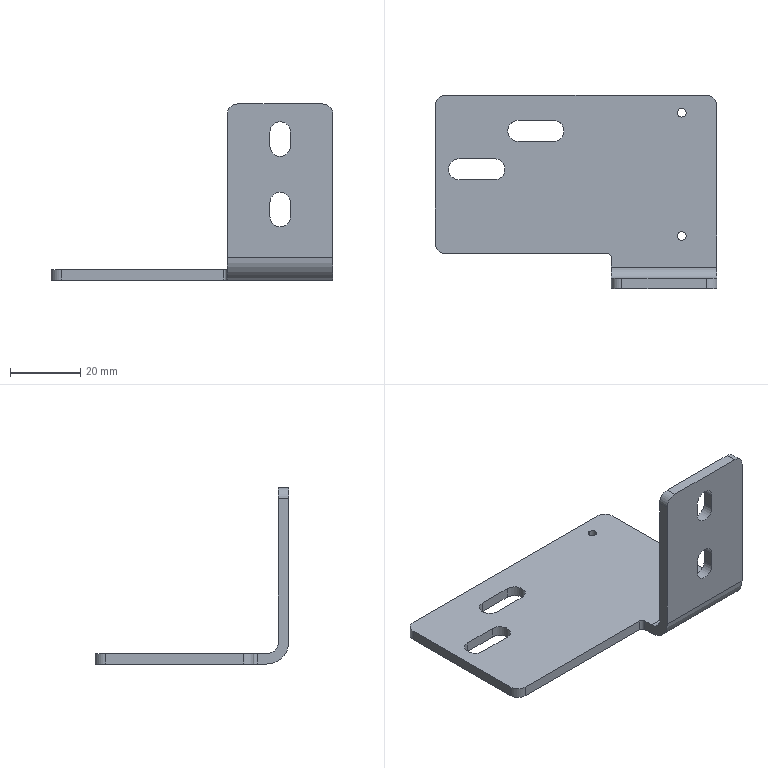Part | STEP file | J014-EBZ05-08-06-Part-1 | 1 solid | 40 faces | box 80 x 55 x 50 mm | volume 14847 mm3 | cylinder 22 | plane 18 | commonest cylinder face diameters 6 x9 5.8 x6 2.5 x4 2 x1 6.4 x1 12.8 x1
STEP:
#1=CARTESIAN_POINT('',(70.,48.75,0.));
#2=VERTEX_POINT('',#1);
#3=CARTESIAN_POINT('',(70.,51.25,0.));
#4=VERTEX_POINT('',#3);
#5=CARTESIAN_POINT('',(70.,50.,0.));
#6=DIRECTION('',(0.,0.,1.));
#7=DIRECTION('',(0.,1.,0.));
#8=AXIS2_PLACEMENT_3D('',#5,#6,#7);
#9=CIRCLE('',#8,1.25);
#10=EDGE_CURVE('',#2,#4,#9,.T.);
#11=ORIENTED_EDGE('',*,*,#10,.F.);
#12=CARTESIAN_POINT('',(70.,48.75,3.));
#13=VERTEX_POINT('',#12);
#14=CARTESIAN_POINT('',(70.,48.75,0.));
#15=DIRECTION('',(0.,0.,1.));
#16=VECTOR('',#15,1000.);
#17=LINE('',#14,#16);
#18=EDGE_CURVE('',#2,#13,#17,.T.);
#19=ORIENTED_EDGE('',*,*,#18,.T.);
#20=CARTESIAN_POINT('',(70.,51.25,3.));
#21=VERTEX_POINT('',#20);
#22=CARTESIAN_POINT('',(70.,50.,3.));
#23=DIRECTION('',(0.,0.,-1.));
#24=DIRECTION('',(0.,-1.,0.));
#25=AXIS2_PLACEMENT_3D('',#22,#23,#24);
#26=CIRCLE('',#25,1.25);
#27=EDGE_CURVE('',#21,#13,#26,.T.);
#28=ORIENTED_EDGE('',*,*,#27,.F.);
#29=CARTESIAN_POINT('',(70.,51.25,0.));
#30=DIRECTION('',(0.,0.,1.));
#31=VECTOR('',#30,1000.);
#32=LINE('',#29,#31);
#33=EDGE_CURVE('',#4,#21,#32,.T.);
#34=ORIENTED_EDGE('',*,*,#33,.F.);
#35=EDGE_LOOP('',(#11,#19,#28,#34));
#36=FACE_OUTER_BOUND('',#35,.T.);
#37=CARTESIAN_POINT('',(70.,50.,0.));
#38=DIRECTION('',(0.,0.,1.));
#39=DIRECTION('',(0.,1.,0.));
#40=AXIS2_PLACEMENT_3D('',#37,#38,#39);
#41=CYLINDRICAL_SURFACE('',#40,1.25);
#42=ADVANCED_FACE('',(#36),#41,.F.);
#43=CARTESIAN_POINT('',(70.,13.75,0.));
#44=VERTEX_POINT('',#43);
#45=CARTESIAN_POINT('',(70.,16.25,0.));
#46=VERTEX_POINT('',#45);
#47=CARTESIAN_POINT('',(70.,15.,0.));
#48=DIRECTION('',(0.,0.,1.));
#49=DIRECTION('',(0.,1.,0.));
#50=AXIS2_PLACEMENT_3D('',#47,#48,#49);
#51=CIRCLE('',#50,1.25);
#52=EDGE_CURVE('',#44,#46,#51,.T.);
#53=ORIENTED_EDGE('',*,*,#52,.F.);
#54=CARTESIAN_POINT('',(70.,13.75,3.));
#55=VERTEX_POINT('',#54);
#56=CARTESIAN_POINT('',(70.,13.75,0.));
#57=DIRECTION('',(0.,0.,1.));
#58=VECTOR('',#57,1000.);
#59=LINE('',#56,#58);
#60=EDGE_CURVE('',#44,#55,#59,.T.);
#61=ORIENTED_EDGE('',*,*,#60,.T.);
#62=CARTESIAN_POINT('',(70.,16.25,3.));
#63=VERTEX_POINT('',#62);
#64=CARTESIAN_POINT('',(70.,15.,3.));
#65=DIRECTION('',(0.,0.,-1.));
#66=DIRECTION('',(0.,-1.,0.));
#67=AXIS2_PLACEMENT_3D('',#64,#65,#66);
#68=CIRCLE('',#67,1.25);
#69=EDGE_CURVE('',#63,#55,#68,.T.);
#70=ORIENTED_EDGE('',*,*,#69,.F.);
#71=CARTESIAN_POINT('',(70.,16.25,0.));
#72=DIRECTION('',(0.,0.,1.));
#73=VECTOR('',#72,1000.);
#74=LINE('',#71,#73);
#75=EDGE_CURVE('',#46,#63,#74,.T.);
#76=ORIENTED_EDGE('',*,*,#75,.F.);
#77=EDGE_LOOP('',(#53,#61,#70,#76));
#78=FACE_OUTER_BOUND('',#77,.T.);
#79=CARTESIAN_POINT('',(70.,15.,0.));
#80=DIRECTION('',(0.,0.,1.));
#81=DIRECTION('',(0.,1.,0.));
#82=AXIS2_PLACEMENT_3D('',#79,#80,#81);
#83=CYLINDRICAL_SURFACE('',#82,1.25);
#84=ADVANCED_FACE('',(#78),#83,.F.);
#85=CARTESIAN_POINT('',(65.,3.,44.9));
#86=VERTEX_POINT('',#85);
#87=CARTESIAN_POINT('',(62.1,3.,42.));
#88=VERTEX_POINT('',#87);
#89=CARTESIAN_POINT('',(65.,3.,42.));
#90=DIRECTION('',(0.,-1.,0.));
#91=DIRECTION('',(0.,0.,1.));
#92=AXIS2_PLACEMENT_3D('',#89,#90,#91);
#93=CIRCLE('',#92,2.9);
#94=EDGE_CURVE('',#86,#88,#93,.T.);
#95=ORIENTED_EDGE('',*,*,#94,.F.);
#96=CARTESIAN_POINT('',(65.,0.,44.9));
#97=VERTEX_POINT('',#96);
#98=CARTESIAN_POINT('',(65.,3.,44.9));
#99=DIRECTION('',(0.,-1.,0.));
#100=VECTOR('',#99,1000.);
#101=LINE('',#98,#100);
#102=EDGE_CURVE('',#86,#97,#101,.T.);
#103=ORIENTED_EDGE('',*,*,#102,.T.);
#104=CARTESIAN_POINT('',(62.1,0.,42.));
#105=VERTEX_POINT('',#104);
#106=CARTESIAN_POINT('',(65.,0.,42.));
#107=DIRECTION('',(0.,1.,0.));
#108=DIRECTION('',(0.,0.,-1.));
#109=AXIS2_PLACEMENT_3D('',#106,#107,#108);
#110=CIRCLE('',#109,2.9);
#111=EDGE_CURVE('',#105,#97,#110,.T.);
#112=ORIENTED_EDGE('',*,*,#111,.F.);
#113=CARTESIAN_POINT('',(62.1,3.,42.));
#114=DIRECTION('',(0.,-1.,0.));
#115=VECTOR('',#114,1000.);
#116=LINE('',#113,#115);
#117=EDGE_CURVE('',#88,#105,#116,.T.);
#118=ORIENTED_EDGE('',*,*,#117,.F.);
#119=EDGE_LOOP('',(#95,#103,#112,#118));
#120=FACE_OUTER_BOUND('',#119,.T.);
#121=CARTESIAN_POINT('',(65.,3.,42.));
#122=DIRECTION('',(0.,-1.,0.));
#123=DIRECTION('',(0.,0.,1.));
#124=AXIS2_PLACEMENT_3D('',#121,#122,#123);
#125=CYLINDRICAL_SURFACE('',#124,2.9);
#126=ADVANCED_FACE('',(#120),#125,.F.);
#127=CARTESIAN_POINT('',(65.,3.,24.9));
#128=VERTEX_POINT('',#127);
#129=CARTESIAN_POINT('',(62.1,3.,22.));
#130=VERTEX_POINT('',#129);
#131=CARTESIAN_POINT('',(65.,3.,22.));
#132=DIRECTION('',(0.,-1.,0.));
#133=DIRECTION('',(0.,0.,1.));
#134=AXIS2_PLACEMENT_3D('',#131,#132,#133);
#135=CIRCLE('',#134,2.9);
#136=EDGE_CURVE('',#128,#130,#135,.T.);
#137=ORIENTED_EDGE('',*,*,#136,.F.);
#138=CARTESIAN_POINT('',(65.,0.,24.9));
#139=VERTEX_POINT('',#138);
#140=CARTESIAN_POINT('',(65.,3.,24.9));
#141=DIRECTION('',(0.,-1.,0.));
#142=VECTOR('',#141,1000.);
#143=LINE('',#140,#142);
#144=EDGE_CURVE('',#128,#139,#143,.T.);
#145=ORIENTED_EDGE('',*,*,#144,.T.);
#146=CARTESIAN_POINT('',(62.1,0.,22.));
#147=VERTEX_POINT('',#146);
#148=CARTESIAN_POINT('',(65.,0.,22.));
#149=DIRECTION('',(0.,1.,0.));
#150=DIRECTION('',(0.,0.,-1.));
#151=AXIS2_PLACEMENT_3D('',#148,#149,#150);
#152=CIRCLE('',#151,2.9);
#153=EDGE_CURVE('',#147,#139,#152,.T.);
#154=ORIENTED_EDGE('',*,*,#153,.F.);
#155=CARTESIAN_POINT('',(62.1,3.,22.));
#156=DIRECTION('',(0.,-1.,0.));
#157=VECTOR('',#156,1000.);
#158=LINE('',#155,#157);
#159=EDGE_CURVE('',#130,#147,#158,.T.);
#160=ORIENTED_EDGE('',*,*,#159,.F.);
#161=EDGE_LOOP('',(#137,#145,#154,#160));
#162=FACE_OUTER_BOUND('',#161,.T.);
#163=CARTESIAN_POINT('',(65.,3.,22.));
#164=DIRECTION('',(0.,-1.,0.));
#165=DIRECTION('',(0.,0.,1.));
#166=AXIS2_PLACEMENT_3D('',#163,#164,#165);
#167=CYLINDRICAL_SURFACE('',#166,2.9);
#168=ADVANCED_FACE('',(#162),#167,.F.);
#169=CARTESIAN_POINT('',(70.,50.,0.));
#170=DIRECTION('',(0.,0.,1.));
#171=DIRECTION('',(0.,1.,0.));
#172=AXIS2_PLACEMENT_3D('',#169,#170,#171);
#173=CIRCLE('',#172,1.25);
#174=EDGE_CURVE('',#4,#2,#173,.T.);
#175=ORIENTED_EDGE('',*,*,#174,.T.);
#176=ORIENTED_EDGE('',*,*,#10,.T.);
#177=EDGE_LOOP('',(#175,#176));
#178=FACE_BOUND('',#177,.T.);
#179=CARTESIAN_POINT('',(70.,15.,0.));
#180=DIRECTION('',(0.,0.,1.));
#181=DIRECTION('',(0.,1.,0.));
#182=AXIS2_PLACEMENT_3D('',#179,#180,#181);
#183=CIRCLE('',#182,1.25);
#184=EDGE_CURVE('',#46,#44,#183,.T.);
#185=ORIENTED_EDGE('',*,*,#184,.T.);
#186=ORIENTED_EDGE('',*,*,#52,.T.);
#187=EDGE_LOOP('',(#185,#186));
#188=FACE_BOUND('',#187,.T.);
#189=CARTESIAN_POINT('',(50.,9.,0.));
#190=VERTEX_POINT('',#189);
#191=CARTESIAN_POINT('',(50.,6.4,0.));
#192=VERTEX_POINT('',#191);
#193=CARTESIAN_POINT('',(50.,3.,0.));
#194=DIRECTION('',(0.,-1.,0.));
#195=VECTOR('',#194,1000.);
#196=LINE('',#193,#195);
#197=EDGE_CURVE('',#190,#192,#196,.T.);
#198=ORIENTED_EDGE('',*,*,#197,.F.);
#199=CARTESIAN_POINT('',(49.,10.,0.));
#200=VERTEX_POINT('',#199);
#201=CARTESIAN_POINT('',(49.,9.,0.));
#202=DIRECTION('',(0.,0.,1.));
#203=DIRECTION('',(0.,-1.,0.));
#204=AXIS2_PLACEMENT_3D('',#201,#202,#203);
#205=CIRCLE('',#204,1.);
#206=EDGE_CURVE('',#190,#200,#205,.T.);
#207=ORIENTED_EDGE('',*,*,#206,.T.);
#208=CARTESIAN_POINT('',(3.,10.,0.));
#209=VERTEX_POINT('',#208);
#210=CARTESIAN_POINT('',(45.,10.,0.));
#211=DIRECTION('',(-1.,0.,0.));
#212=VECTOR('',#211,1000.);
#213=LINE('',#210,#212);
#214=EDGE_CURVE('',#200,#209,#213,.T.);
#215=ORIENTED_EDGE('',*,*,#214,.T.);
#216=CARTESIAN_POINT('',(0.,13.,0.));
#217=VERTEX_POINT('',#216);
#218=CARTESIAN_POINT('',(3.,13.,0.));
#219=DIRECTION('',(0.,0.,-1.));
#220=DIRECTION('',(0.,-1.,0.));
#221=AXIS2_PLACEMENT_3D('',#218,#219,#220);
#222=CIRCLE('',#221,3.);
#223=EDGE_CURVE('',#209,#217,#222,.T.);
#224=ORIENTED_EDGE('',*,*,#223,.T.);
#225=CARTESIAN_POINT('',(0.,52.,0.));
#226=VERTEX_POINT('',#225);
#227=CARTESIAN_POINT('',(0.,27.5,0.));
#228=DIRECTION('',(0.,-1.,0.));
#229=VECTOR('',#228,1000.);
#230=LINE('',#227,#229);
#231=EDGE_CURVE('',#226,#217,#230,.T.);
#232=ORIENTED_EDGE('',*,*,#231,.F.);
#233=CARTESIAN_POINT('',(3.,55.,0.));
#234=VERTEX_POINT('',#233);
#235=CARTESIAN_POINT('',(3.,52.,0.));
#236=DIRECTION('',(0.,0.,-1.));
#237=DIRECTION('',(0.,-1.,0.));
#238=AXIS2_PLACEMENT_3D('',#235,#236,#237);
#239=CIRCLE('',#238,3.);
#240=EDGE_CURVE('',#226,#234,#239,.T.);
#241=ORIENTED_EDGE('',*,*,#240,.T.);
#242=CARTESIAN_POINT('',(77.,55.,0.));
#243=VERTEX_POINT('',#242);
#244=CARTESIAN_POINT('',(40.,55.,0.));
#245=DIRECTION('',(-1.,0.,0.));
#246=VECTOR('',#245,1000.);
#247=LINE('',#244,#246);
#248=EDGE_CURVE('',#243,#234,#247,.T.);
#249=ORIENTED_EDGE('',*,*,#248,.F.);
#250=CARTESIAN_POINT('',(80.,52.,0.));
#251=VERTEX_POINT('',#250);
#252=CARTESIAN_POINT('',(77.,52.,0.));
#253=DIRECTION('',(0.,0.,-1.));
#254=DIRECTION('',(0.,-1.,0.));
#255=AXIS2_PLACEMENT_3D('',#252,#253,#254);
#256=CIRCLE('',#255,3.);
#257=EDGE_CURVE('',#243,#251,#256,.T.);
#258=ORIENTED_EDGE('',*,*,#257,.T.);
#259=CARTESIAN_POINT('',(80.,6.4,0.));
#260=VERTEX_POINT('',#259);
#261=CARTESIAN_POINT('',(80.,3.,0.));
#262=DIRECTION('',(0.,-1.,0.));
#263=VECTOR('',#262,1000.);
#264=LINE('',#261,#263);
#265=EDGE_CURVE('',#251,#260,#264,.T.);
#266=ORIENTED_EDGE('',*,*,#265,.T.);
#267=CARTESIAN_POINT('',(65.,6.4,0.));
#268=DIRECTION('',(-1.,0.,0.));
#269=VECTOR('',#268,1000.);
#270=LINE('',#267,#269);
#271=EDGE_CURVE('',#260,#192,#270,.T.);
#272=ORIENTED_EDGE('',*,*,#271,.T.);
#273=EDGE_LOOP('',(#198,#207,#215,#224,#232,#241,#249,#258,#266,#272));
#274=FACE_OUTER_BOUND('',#273,.T.);
#275=CARTESIAN_POINT('',(23.604,41.839,0.));
#276=VERTEX_POINT('',#275);
#277=CARTESIAN_POINT('',(33.604,41.839,0.));
#278=VERTEX_POINT('',#277);
#279=CARTESIAN_POINT('',(28.604,41.839,0.));
#280=DIRECTION('',(1.,0.,0.));
#281=VECTOR('',#280,1000.);
#282=LINE('',#279,#281);
#283=EDGE_CURVE('',#276,#278,#282,.T.);
#284=ORIENTED_EDGE('',*,*,#283,.T.);
#285=CARTESIAN_POINT('',(33.604,47.839,0.));
#286=VERTEX_POINT('',#285);
#287=CARTESIAN_POINT('',(33.604,44.839,0.));
#288=DIRECTION('',(0.,0.,1.));
#289=DIRECTION('',(0.,1.,0.));
#290=AXIS2_PLACEMENT_3D('',#287,#288,#289);
#291=CIRCLE('',#290,3.);
#292=EDGE_CURVE('',#278,#286,#291,.T.);
#293=ORIENTED_EDGE('',*,*,#292,.T.);
#294=CARTESIAN_POINT('',(23.604,47.839,0.));
#295=VERTEX_POINT('',#294);
#296=CARTESIAN_POINT('',(28.604,47.839,0.));
#297=DIRECTION('',(-1.,0.,0.));
#298=VECTOR('',#297,1000.);
#299=LINE('',#296,#298);
#300=EDGE_CURVE('',#286,#295,#299,.T.);
#301=ORIENTED_EDGE('',*,*,#300,.T.);
#302=CARTESIAN_POINT('',(23.604,44.839,0.));
#303=DIRECTION('',(0.,0.,1.));
#304=DIRECTION('',(0.,1.,0.));
#305=AXIS2_PLACEMENT_3D('',#302,#303,#304);
#306=CIRCLE('',#305,3.);
#307=EDGE_CURVE('',#295,#276,#306,.T.);
#308=ORIENTED_EDGE('',*,*,#307,.T.);
#309=EDGE_LOOP('',(#284,#293,#301,#308));
#310=FACE_BOUND('',#309,.T.);
#311=CARTESIAN_POINT('',(6.831,30.947,0.));
#312=VERTEX_POINT('',#311);
#313=CARTESIAN_POINT('',(16.831,30.947,0.));
#314=VERTEX_POINT('',#313);
#315=CARTESIAN_POINT('',(11.831,30.947,0.));
#316=DIRECTION('',(1.,0.,0.));
#317=VECTOR('',#316,1000.);
#318=LINE('',#315,#317);
#319=EDGE_CURVE('',#312,#314,#318,.T.);
#320=ORIENTED_EDGE('',*,*,#319,.T.);
#321=CARTESIAN_POINT('',(16.831,36.947,0.));
#322=VERTEX_POINT('',#321);
#323=CARTESIAN_POINT('',(16.831,33.947,0.));
#324=DIRECTION('',(0.,0.,1.));
#325=DIRECTION('',(0.,1.,0.));
#326=AXIS2_PLACEMENT_3D('',#323,#324,#325);
#327=CIRCLE('',#326,3.);
#328=EDGE_CURVE('',#314,#322,#327,.T.);
#329=ORIENTED_EDGE('',*,*,#328,.T.);
#330=CARTESIAN_POINT('',(6.831,36.947,0.));
#331=VERTEX_POINT('',#330);
#332=CARTESIAN_POINT('',(11.831,36.947,0.));
#333=DIRECTION('',(-1.,0.,0.));
#334=VECTOR('',#333,1000.);
#335=LINE('',#332,#334);
#336=EDGE_CURVE('',#322,#331,#335,.T.);
#337=ORIENTED_EDGE('',*,*,#336,.T.);
#338=CARTESIAN_POINT('',(6.831,33.947,0.));
#339=DIRECTION('',(0.,0.,1.));
#340=DIRECTION('',(0.,1.,0.));
#341=AXIS2_PLACEMENT_3D('',#338,#339,#340);
#342=CIRCLE('',#341,3.);
#343=EDGE_CURVE('',#331,#312,#342,.T.);
#344=ORIENTED_EDGE('',*,*,#343,.T.);
#345=EDGE_LOOP('',(#320,#329,#337,#344));
#346=FACE_BOUND('',#345,.T.);
#347=CARTESIAN_POINT('',(65.,3.,0.));
#348=DIRECTION('',(0.,0.,-1.));
#349=DIRECTION('',(0.,-1.,0.));
#350=AXIS2_PLACEMENT_3D('',#347,#348,#349);
#351=PLANE('',#350);
#352=ADVANCED_FACE('',(#178,#188,#274,#310,#346),#351,.T.);
#353=CARTESIAN_POINT('',(80.,0.,47.));
#354=VERTEX_POINT('',#353);
#355=CARTESIAN_POINT('',(80.,0.,6.4));
#356=VERTEX_POINT('',#355);
#357=CARTESIAN_POINT('',(80.,0.,25.));
#358=DIRECTION('',(0.,0.,-1.));
#359=VECTOR('',#358,1000.);
#360=LINE('',#357,#359);
#361=EDGE_CURVE('',#354,#356,#360,.T.);
#362=ORIENTED_EDGE('',*,*,#361,.F.);
#363=CARTESIAN_POINT('',(77.,0.,50.));
#364=VERTEX_POINT('',#363);
#365=CARTESIAN_POINT('',(77.,0.,47.));
#366=DIRECTION('',(0.,-1.,0.));
#367=DIRECTION('',(-1.,0.,0.));
#368=AXIS2_PLACEMENT_3D('',#365,#366,#367);
#369=CIRCLE('',#368,3.);
#370=EDGE_CURVE('',#354,#364,#369,.T.);
#371=ORIENTED_EDGE('',*,*,#370,.T.);
#372=CARTESIAN_POINT('',(53.,0.,50.));
#373=VERTEX_POINT('',#372);
#374=CARTESIAN_POINT('',(65.,0.,50.));
#375=DIRECTION('',(1.,0.,0.));
#376=VECTOR('',#375,1000.);
#377=LINE('',#374,#376);
#378=EDGE_CURVE('',#373,#364,#377,.T.);
#379=ORIENTED_EDGE('',*,*,#378,.F.);
#380=CARTESIAN_POINT('',(50.,0.,47.));
#381=VERTEX_POINT('',#380);
#382=CARTESIAN_POINT('',(53.,0.,47.));
#383=DIRECTION('',(0.,-1.,0.));
#384=DIRECTION('',(-1.,0.,0.));
#385=AXIS2_PLACEMENT_3D('',#382,#383,#384);
#386=CIRCLE('',#385,3.);
#387=EDGE_CURVE('',#373,#381,#386,.T.);
#388=ORIENTED_EDGE('',*,*,#387,.T.);
#389=CARTESIAN_POINT('',(50.,0.,6.4));
#390=VERTEX_POINT('',#389);
#391=CARTESIAN_POINT('',(50.,0.,25.));
#392=DIRECTION('',(0.,0.,1.));
#393=VECTOR('',#392,1000.);
#394=LINE('',#391,#393);
#395=EDGE_CURVE('',#390,#381,#394,.T.);
#396=ORIENTED_EDGE('',*,*,#395,.F.);
#397=CARTESIAN_POINT('',(65.,0.,6.4));
#398=DIRECTION('',(1.,0.,0.));
#399=VECTOR('',#398,1000.);
#400=LINE('',#397,#399);
#401=EDGE_CURVE('',#390,#356,#400,.T.);
#402=ORIENTED_EDGE('',*,*,#401,.T.);
#403=EDGE_LOOP('',(#362,#371,#379,#388,#396,#402));
#404=FACE_OUTER_BOUND('',#403,.T.);
#405=CARTESIAN_POINT('',(62.1,0.,18.));
#406=VERTEX_POINT('',#405);
#407=CARTESIAN_POINT('',(62.1,0.,20.));
#408=DIRECTION('',(0.,0.,1.));
#409=VECTOR('',#408,1000.);
#410=LINE('',#407,#409);
#411=EDGE_CURVE('',#406,#147,#410,.T.);
#412=ORIENTED_EDGE('',*,*,#411,.T.);
#413=ORIENTED_EDGE('',*,*,#153,.T.);
#414=CARTESIAN_POINT('',(67.9,0.,22.));
#415=VERTEX_POINT('',#414);
#416=CARTESIAN_POINT('',(65.,0.,22.));
#417=DIRECTION('',(0.,1.,0.));
#418=DIRECTION('',(0.,0.,-1.));
#419=AXIS2_PLACEMENT_3D('',#416,#417,#418);
#420=CIRCLE('',#419,2.9);
#421=EDGE_CURVE('',#139,#415,#420,.T.);
#422=ORIENTED_EDGE('',*,*,#421,.T.);
#423=CARTESIAN_POINT('',(67.9,0.,18.));
#424=VERTEX_POINT('',#423);
#425=CARTESIAN_POINT('',(67.9,0.,20.));
#426=DIRECTION('',(0.,0.,-1.));
#427=VECTOR('',#426,1000.);
#428=LINE('',#425,#427);
#429=EDGE_CURVE('',#415,#424,#428,.T.);
#430=ORIENTED_EDGE('',*,*,#429,.T.);
#431=CARTESIAN_POINT('',(65.,0.,18.));
#432=DIRECTION('',(0.,1.,0.));
#433=DIRECTION('',(0.,0.,-1.));
#434=AXIS2_PLACEMENT_3D('',#431,#432,#433);
#435=CIRCLE('',#434,2.9);
#436=EDGE_CURVE('',#424,#406,#435,.T.);
#437=ORIENTED_EDGE('',*,*,#436,.T.);
#438=EDGE_LOOP('',(#412,#413,#422,#430,#437));
#439=FACE_BOUND('',#438,.T.);
#440=CARTESIAN_POINT('',(62.1,0.,38.));
#441=VERTEX_POINT('',#440);
#442=CARTESIAN_POINT('',(62.1,0.,40.));
#443=DIRECTION('',(0.,0.,1.));
#444=VECTOR('',#443,1000.);
#445=LINE('',#442,#444);
#446=EDGE_CURVE('',#441,#105,#445,.T.);
#447=ORIENTED_EDGE('',*,*,#446,.T.);
#448=ORIENTED_EDGE('',*,*,#111,.T.);
#449=CARTESIAN_POINT('',(67.9,0.,42.));
#450=VERTEX_POINT('',#449);
#451=CARTESIAN_POINT('',(65.,0.,42.));
#452=DIRECTION('',(0.,1.,0.));
#453=DIRECTION('',(0.,0.,-1.));
#454=AXIS2_PLACEMENT_3D('',#451,#452,#453);
#455=CIRCLE('',#454,2.9);
#456=EDGE_CURVE('',#97,#450,#455,.T.);
#457=ORIENTED_EDGE('',*,*,#456,.T.);
#458=CARTESIAN_POINT('',(67.9,0.,38.));
#459=VERTEX_POINT('',#458);
#460=CARTESIAN_POINT('',(67.9,0.,40.));
#461=DIRECTION('',(0.,0.,-1.));
#462=VECTOR('',#461,1000.);
#463=LINE('',#460,#462);
#464=EDGE_CURVE('',#450,#459,#463,.T.);
#465=ORIENTED_EDGE('',*,*,#464,.T.);
#466=CARTESIAN_POINT('',(65.,0.,38.));
#467=DIRECTION('',(0.,1.,0.));
#468=DIRECTION('',(0.,0.,-1.));
#469=AXIS2_PLACEMENT_3D('',#466,#467,#468);
#470=CIRCLE('',#469,2.9);
#471=EDGE_CURVE('',#459,#441,#470,.T.);
#472=ORIENTED_EDGE('',*,*,#471,.T.);
#473=EDGE_LOOP('',(#447,#448,#457,#465,#472));
#474=FACE_BOUND('',#473,.T.);
#475=CARTESIAN_POINT('',(65.,0.,25.));
#476=DIRECTION('',(0.,-1.,0.));
#477=DIRECTION('',(-1.,0.,0.));
#478=AXIS2_PLACEMENT_3D('',#475,#476,#477);
#479=PLANE('',#478);
#480=ADVANCED_FACE('',(#404,#439,#474),#479,.T.);
#481=CARTESIAN_POINT('',(77.,3.,50.));
#482=VERTEX_POINT('',#481);
#483=CARTESIAN_POINT('',(53.,3.,50.));
#484=VERTEX_POINT('',#483);
#485=CARTESIAN_POINT('',(65.,3.,50.));
#486=DIRECTION('',(-1.,0.,0.));
#487=VECTOR('',#486,1000.);
#488=LINE('',#485,#487);
#489=EDGE_CURVE('',#482,#484,#488,.T.);
#490=ORIENTED_EDGE('',*,*,#489,.F.);
#491=CARTESIAN_POINT('',(80.,3.,47.));
#492=VERTEX_POINT('',#491);
#493=CARTESIAN_POINT('',(77.,3.,47.));
#494=DIRECTION('',(0.,1.,0.));
#495=DIRECTION('',(1.,0.,0.));
#496=AXIS2_PLACEMENT_3D('',#493,#494,#495);
#497=CIRCLE('',#496,3.);
#498=EDGE_CURVE('',#482,#492,#497,.T.);
#499=ORIENTED_EDGE('',*,*,#498,.T.);
#500=CARTESIAN_POINT('',(80.,3.,6.2));
#501=VERTEX_POINT('',#500);
#502=CARTESIAN_POINT('',(80.,3.,25.));
#503=DIRECTION('',(0.,0.,1.));
#504=VECTOR('',#503,1000.);
#505=LINE('',#502,#504);
#506=EDGE_CURVE('',#501,#492,#505,.T.);
#507=ORIENTED_EDGE('',*,*,#506,.F.);
#508=CARTESIAN_POINT('',(50.,3.,6.2));
#509=VERTEX_POINT('',#508);
#510=CARTESIAN_POINT('',(50.,3.,6.2));
#511=DIRECTION('',(-1.,0.,0.));
#512=VECTOR('',#511,1000.);
#513=LINE('',#510,#512);
#514=EDGE_CURVE('',#501,#509,#513,.T.);
#515=ORIENTED_EDGE('',*,*,#514,.T.);
#516=CARTESIAN_POINT('',(50.,3.,47.));
#517=VERTEX_POINT('',#516);
#518=CARTESIAN_POINT('',(50.,3.,25.));
#519=DIRECTION('',(0.,0.,-1.));
#520=VECTOR('',#519,1000.);
#521=LINE('',#518,#520);
#522=EDGE_CURVE('',#517,#509,#521,.T.);
#523=ORIENTED_EDGE('',*,*,#522,.F.);
#524=CARTESIAN_POINT('',(53.,3.,47.));
#525=DIRECTION('',(0.,1.,0.));
#526=DIRECTION('',(1.,0.,0.));
#527=AXIS2_PLACEMENT_3D('',#524,#525,#526);
#528=CIRCLE('',#527,3.);
#529=EDGE_CURVE('',#517,#484,#528,.T.);
#530=ORIENTED_EDGE('',*,*,#529,.T.);
#531=EDGE_LOOP('',(#490,#499,#507,#515,#523,#530));
#532=FACE_OUTER_BOUND('',#531,.T.);
#533=CARTESIAN_POINT('',(67.9,3.,18.));
#534=VERTEX_POINT('',#533);
#535=CARTESIAN_POINT('',(67.9,3.,22.));
#536=VERTEX_POINT('',#535);
#537=CARTESIAN_POINT('',(67.9,3.,20.));
#538=DIRECTION('',(0.,0.,1.));
#539=VECTOR('',#538,1000.);
#540=LINE('',#537,#539);
#541=EDGE_CURVE('',#534,#536,#540,.T.);
#542=ORIENTED_EDGE('',*,*,#541,.T.);
#543=CARTESIAN_POINT('',(65.,3.,22.));
#544=DIRECTION('',(0.,-1.,0.));
#545=DIRECTION('',(0.,0.,1.));
#546=AXIS2_PLACEMENT_3D('',#543,#544,#545);
#547=CIRCLE('',#546,2.9);
#548=EDGE_CURVE('',#536,#128,#547,.T.);
#549=ORIENTED_EDGE('',*,*,#548,.T.);
#550=ORIENTED_EDGE('',*,*,#136,.T.);
#551=CARTESIAN_POINT('',(62.1,3.,18.));
#552=VERTEX_POINT('',#551);
#553=CARTESIAN_POINT('',(62.1,3.,20.));
#554=DIRECTION('',(0.,0.,-1.));
#555=VECTOR('',#554,1000.);
#556=LINE('',#553,#555);
#557=EDGE_CURVE('',#130,#552,#556,.T.);
#558=ORIENTED_EDGE('',*,*,#557,.T.);
#559=CARTESIAN_POINT('',(65.,3.,18.));
#560=DIRECTION('',(0.,-1.,0.));
#561=DIRECTION('',(0.,0.,1.));
#562=AXIS2_PLACEMENT_3D('',#559,#560,#561);
#563=CIRCLE('',#562,2.9);
#564=EDGE_CURVE('',#552,#534,#563,.T.);
#565=ORIENTED_EDGE('',*,*,#564,.T.);
#566=EDGE_LOOP('',(#542,#549,#550,#558,#565));
#567=FACE_BOUND('',#566,.T.);
#568=CARTESIAN_POINT('',(67.9,3.,38.));
#569=VERTEX_POINT('',#568);
#570=CARTESIAN_POINT('',(67.9,3.,42.));
#571=VERTEX_POINT('',#570);
#572=CARTESIAN_POINT('',(67.9,3.,40.));
#573=DIRECTION('',(0.,0.,1.));
#574=VECTOR('',#573,1000.);
#575=LINE('',#572,#574);
#576=EDGE_CURVE('',#569,#571,#575,.T.);
#577=ORIENTED_EDGE('',*,*,#576,.T.);
#578=CARTESIAN_POINT('',(65.,3.,42.));
#579=DIRECTION('',(0.,-1.,0.));
#580=DIRECTION('',(0.,0.,1.));
#581=AXIS2_PLACEMENT_3D('',#578,#579,#580);
#582=CIRCLE('',#581,2.9);
#583=EDGE_CURVE('',#571,#86,#582,.T.);
#584=ORIENTED_EDGE('',*,*,#583,.T.);
#585=ORIENTED_EDGE('',*,*,#94,.T.);
#586=CARTESIAN_POINT('',(62.1,3.,38.));
#587=VERTEX_POINT('',#586);
#588=CARTESIAN_POINT('',(62.1,3.,40.));
#589=DIRECTION('',(0.,0.,-1.));
#590=VECTOR('',#589,1000.);
#591=LINE('',#588,#590);
#592=EDGE_CURVE('',#88,#587,#591,.T.);
#593=ORIENTED_EDGE('',*,*,#592,.T.);
#594=CARTESIAN_POINT('',(65.,3.,38.));
#595=DIRECTION('',(0.,-1.,0.));
#596=DIRECTION('',(0.,0.,1.));
#597=AXIS2_PLACEMENT_3D('',#594,#595,#596);
#598=CIRCLE('',#597,2.9);
#599=EDGE_CURVE('',#587,#569,#598,.T.);
#600=ORIENTED_EDGE('',*,*,#599,.T.);
#601=EDGE_LOOP('',(#577,#584,#585,#593,#600));
#602=FACE_BOUND('',#601,.T.);
#603=CARTESIAN_POINT('',(65.,3.,25.));
#604=DIRECTION('',(0.,1.,0.));
#605=DIRECTION('',(1.,0.,0.));
#606=AXIS2_PLACEMENT_3D('',#603,#604,#605);
#607=PLANE('',#606);
#608=ADVANCED_FACE('',(#532,#567,#602),#607,.T.);
#609=ORIENTED_EDGE('',*,*,#378,.T.);
#610=CARTESIAN_POINT('',(77.,3.,50.));
#611=DIRECTION('',(0.,1.,0.));
#612=VECTOR('',#611,1000.);
#613=LINE('',#610,#612);
#614=EDGE_CURVE('',#364,#482,#613,.T.);
#615=ORIENTED_EDGE('',*,*,#614,.T.);
#616=ORIENTED_EDGE('',*,*,#489,.T.);
#617=CARTESIAN_POINT('',(53.,3.,50.));
#618=DIRECTION('',(0.,-1.,0.));
#619=VECTOR('',#618,1000.);
#620=LINE('',#617,#619);
#621=EDGE_CURVE('',#484,#373,#620,.T.);
#622=ORIENTED_EDGE('',*,*,#621,.T.);
#623=EDGE_LOOP('',(#609,#615,#616,#622));
#624=FACE_OUTER_BOUND('',#623,.T.);
#625=CARTESIAN_POINT('',(65.,3.,50.));
#626=DIRECTION('',(0.,0.,1.));
#627=DIRECTION('',(0.,1.,0.));
#628=AXIS2_PLACEMENT_3D('',#625,#626,#627);
#629=PLANE('',#628);
#630=ADVANCED_FACE('',(#624),#629,.T.);
#631=ORIENTED_EDGE('',*,*,#265,.F.);
#632=CARTESIAN_POINT('',(80.,52.,3.));
#633=VERTEX_POINT('',#632);
#634=CARTESIAN_POINT('',(80.,52.,25.));
#635=DIRECTION('',(0.,0.,1.));
#636=VECTOR('',#635,1000.);
#637=LINE('',#634,#636);
#638=EDGE_CURVE('',#251,#633,#637,.T.);
#639=ORIENTED_EDGE('',*,*,#638,.T.);
#640=CARTESIAN_POINT('',(80.,6.2,3.));
#641=VERTEX_POINT('',#640);
#642=CARTESIAN_POINT('',(80.,27.5,3.));
#643=DIRECTION('',(0.,-1.,0.));
#644=VECTOR('',#643,1000.);
#645=LINE('',#642,#644);
#646=EDGE_CURVE('',#633,#641,#645,.T.);
#647=ORIENTED_EDGE('',*,*,#646,.T.);
#648=CARTESIAN_POINT('',(80.,6.2,6.2));
#649=DIRECTION('',(-1.,0.,0.));
#650=DIRECTION('',(0.,-1.,0.));
#651=AXIS2_PLACEMENT_3D('',#648,#649,#650);
#652=CIRCLE('',#651,3.2);
#653=EDGE_CURVE('',#641,#501,#652,.T.);
#654=ORIENTED_EDGE('',*,*,#653,.T.);
#655=ORIENTED_EDGE('',*,*,#506,.T.);
#656=CARTESIAN_POINT('',(80.,3.,47.));
#657=DIRECTION('',(0.,-1.,0.));
#658=VECTOR('',#657,1000.);
#659=LINE('',#656,#658);
#660=EDGE_CURVE('',#492,#354,#659,.T.);
#661=ORIENTED_EDGE('',*,*,#660,.T.);
#662=ORIENTED_EDGE('',*,*,#361,.T.);
#663=CARTESIAN_POINT('',(80.,6.4,6.4));
#664=DIRECTION('',(1.,0.,0.));
#665=DIRECTION('',(0.,-1.,0.));
#666=AXIS2_PLACEMENT_3D('',#663,#664,#665);
#667=CIRCLE('',#666,6.4);
#668=EDGE_CURVE('',#356,#260,#667,.T.);
#669=ORIENTED_EDGE('',*,*,#668,.T.);
#670=EDGE_LOOP('',(#631,#639,#647,#654,#655,#661,#662,#669));
#671=FACE_OUTER_BOUND('',#670,.T.);
#672=CARTESIAN_POINT('',(80.,3.,25.));
#673=DIRECTION('',(1.,0.,0.));
#674=DIRECTION('',(0.,-1.,0.));
#675=AXIS2_PLACEMENT_3D('',#672,#673,#674);
#676=PLANE('',#675);
#677=ADVANCED_FACE('',(#671),#676,.T.);
#678=CARTESIAN_POINT('',(50.,9.,3.));
#679=VERTEX_POINT('',#678);
#680=CARTESIAN_POINT('',(50.,6.2,3.));
#681=VERTEX_POINT('',#680);
#682=CARTESIAN_POINT('',(50.,5.,3.));
#683=DIRECTION('',(0.,-1.,0.));
#684=VECTOR('',#683,1000.);
#685=LINE('',#682,#684);
#686=EDGE_CURVE('',#679,#681,#685,.T.);
#687=ORIENTED_EDGE('',*,*,#686,.F.);
#688=CARTESIAN_POINT('',(50.,9.,25.));
#689=DIRECTION('',(0.,0.,-1.));
#690=VECTOR('',#689,1000.);
#691=LINE('',#688,#690);
#692=EDGE_CURVE('',#679,#190,#691,.T.);
#693=ORIENTED_EDGE('',*,*,#692,.T.);
#694=ORIENTED_EDGE('',*,*,#197,.T.);
#695=CARTESIAN_POINT('',(50.,6.4,6.4));
#696=DIRECTION('',(-1.,0.,0.));
#697=DIRECTION('',(0.,1.,0.));
#698=AXIS2_PLACEMENT_3D('',#695,#696,#697);
#699=CIRCLE('',#698,6.4);
#700=EDGE_CURVE('',#192,#390,#699,.T.);
#701=ORIENTED_EDGE('',*,*,#700,.T.);
#702=ORIENTED_EDGE('',*,*,#395,.T.);
#703=CARTESIAN_POINT('',(50.,3.,47.));
#704=DIRECTION('',(0.,1.,0.));
#705=VECTOR('',#704,1000.);
#706=LINE('',#703,#705);
#707=EDGE_CURVE('',#381,#517,#706,.T.);
#708=ORIENTED_EDGE('',*,*,#707,.T.);
#709=ORIENTED_EDGE('',*,*,#522,.T.);
#710=CARTESIAN_POINT('',(50.,6.2,6.2));
#711=DIRECTION('',(1.,0.,0.));
#712=DIRECTION('',(0.,1.,0.));
#713=AXIS2_PLACEMENT_3D('',#710,#711,#712);
#714=CIRCLE('',#713,3.2);
#715=EDGE_CURVE('',#509,#681,#714,.T.);
#716=ORIENTED_EDGE('',*,*,#715,.T.);
#717=EDGE_LOOP('',(#687,#693,#694,#701,#702,#708,#709,#716));
#718=FACE_OUTER_BOUND('',#717,.T.);
#719=CARTESIAN_POINT('',(50.,3.,25.));
#720=DIRECTION('',(-1.,0.,0.));
#721=DIRECTION('',(0.,1.,0.));
#722=AXIS2_PLACEMENT_3D('',#719,#720,#721);
#723=PLANE('',#722);
#724=ADVANCED_FACE('',(#718),#723,.T.);
#725=CARTESIAN_POINT('',(16.831,30.947,3.));
#726=VERTEX_POINT('',#725);
#727=CARTESIAN_POINT('',(16.831,36.947,3.));
#728=VERTEX_POINT('',#727);
#729=CARTESIAN_POINT('',(16.831,33.947,3.));
#730=DIRECTION('',(0.,0.,1.));
#731=DIRECTION('',(-1.,0.,0.));
#732=AXIS2_PLACEMENT_3D('',#729,#730,#731);
#733=CIRCLE('',#732,3.);
#734=EDGE_CURVE('',#726,#728,#733,.T.);
#735=ORIENTED_EDGE('',*,*,#734,.F.);
#736=CARTESIAN_POINT('',(6.831,30.947,3.));
#737=VERTEX_POINT('',#736);
#738=CARTESIAN_POINT('',(40.,30.947,3.));
#739=DIRECTION('',(1.,0.,0.));
#740=VECTOR('',#739,1000.);
#741=LINE('',#738,#740);
#742=EDGE_CURVE('',#737,#726,#741,.T.);
#743=ORIENTED_EDGE('',*,*,#742,.F.);
#744=CARTESIAN_POINT('',(6.831,36.947,3.));
#745=VERTEX_POINT('',#744);
#746=CARTESIAN_POINT('',(6.831,33.947,3.));
#747=DIRECTION('',(0.,0.,1.));
#748=DIRECTION('',(-1.,0.,0.));
#749=AXIS2_PLACEMENT_3D('',#746,#747,#748);
#750=CIRCLE('',#749,3.);
#751=EDGE_CURVE('',#745,#737,#750,.T.);
#752=ORIENTED_EDGE('',*,*,#751,.F.);
#753=CARTESIAN_POINT('',(40.,36.947,3.));
#754=DIRECTION('',(-1.,0.,0.));
#755=VECTOR('',#754,1000.);
#756=LINE('',#753,#755);
#757=EDGE_CURVE('',#728,#745,#756,.T.);
#758=ORIENTED_EDGE('',*,*,#757,.F.);
#759=EDGE_LOOP('',(#735,#743,#752,#758));
#760=FACE_BOUND('',#759,.T.);
#761=CARTESIAN_POINT('',(33.604,41.839,3.));
#762=VERTEX_POINT('',#761);
#763=CARTESIAN_POINT('',(33.604,47.839,3.));
#764=VERTEX_POINT('',#763);
#765=CARTESIAN_POINT('',(33.604,44.839,3.));
#766=DIRECTION('',(0.,0.,1.));
#767=DIRECTION('',(-1.,0.,0.));
#768=AXIS2_PLACEMENT_3D('',#765,#766,#767);
#769=CIRCLE('',#768,3.);
#770=EDGE_CURVE('',#762,#764,#769,.T.);
#771=ORIENTED_EDGE('',*,*,#770,.F.);
#772=CARTESIAN_POINT('',(23.604,41.839,3.));
#773=VERTEX_POINT('',#772);
#774=CARTESIAN_POINT('',(40.,41.839,3.));
#775=DIRECTION('',(1.,0.,0.));
#776=VECTOR('',#775,1000.);
#777=LINE('',#774,#776);
#778=EDGE_CURVE('',#773,#762,#777,.T.);
#779=ORIENTED_EDGE('',*,*,#778,.F.);
#780=CARTESIAN_POINT('',(23.604,47.839,3.));
#781=VERTEX_POINT('',#780);
#782=CARTESIAN_POINT('',(23.604,44.839,3.));
#783=DIRECTION('',(0.,0.,1.));
#784=DIRECTION('',(-1.,0.,0.));
#785=AXIS2_PLACEMENT_3D('',#782,#783,#784);
#786=CIRCLE('',#785,3.);
#787=EDGE_CURVE('',#781,#773,#786,.T.);
#788=ORIENTED_EDGE('',*,*,#787,.F.);
#789=CARTESIAN_POINT('',(40.,47.839,3.));
#790=DIRECTION('',(-1.,0.,0.));
#791=VECTOR('',#790,1000.);
#792=LINE('',#789,#791);
#793=EDGE_CURVE('',#764,#781,#792,.T.);
#794=ORIENTED_EDGE('',*,*,#793,.F.);
#795=EDGE_LOOP('',(#771,#779,#788,#794));
#796=FACE_BOUND('',#795,.T.);
#797=ORIENTED_EDGE('',*,*,#27,.T.);
#798=CARTESIAN_POINT('',(70.,50.,3.));
#799=DIRECTION('',(0.,0.,-1.));
#800=DIRECTION('',(0.,-1.,0.));
#801=AXIS2_PLACEMENT_3D('',#798,#799,#800);
#802=CIRCLE('',#801,1.25);
#803=EDGE_CURVE('',#13,#21,#802,.T.);
#804=ORIENTED_EDGE('',*,*,#803,.T.);
#805=EDGE_LOOP('',(#797,#804));
#806=FACE_BOUND('',#805,.T.);
#807=ORIENTED_EDGE('',*,*,#69,.T.);
#808=CARTESIAN_POINT('',(70.,15.,3.));
#809=DIRECTION('',(0.,0.,-1.));
#810=DIRECTION('',(0.,-1.,0.));
#811=AXIS2_PLACEMENT_3D('',#808,#809,#810);
#812=CIRCLE('',#811,1.25);
#813=EDGE_CURVE('',#55,#63,#812,.T.);
#814=ORIENTED_EDGE('',*,*,#813,.T.);
#815=EDGE_LOOP('',(#807,#814));
#816=FACE_BOUND('',#815,.T.);
#817=CARTESIAN_POINT('',(0.,13.,3.));
#818=VERTEX_POINT('',#817);
#819=CARTESIAN_POINT('',(0.,52.,3.));
#820=VERTEX_POINT('',#819);
#821=CARTESIAN_POINT('',(0.,27.5,3.));
#822=DIRECTION('',(0.,1.,0.));
#823=VECTOR('',#822,1000.);
#824=LINE('',#821,#823);
#825=EDGE_CURVE('',#818,#820,#824,.T.);
#826=ORIENTED_EDGE('',*,*,#825,.F.);
#827=CARTESIAN_POINT('',(3.,10.,3.));
#828=VERTEX_POINT('',#827);
#829=CARTESIAN_POINT('',(3.,13.,3.));
#830=DIRECTION('',(0.,0.,1.));
#831=DIRECTION('',(-1.,0.,0.));
#832=AXIS2_PLACEMENT_3D('',#829,#830,#831);
#833=CIRCLE('',#832,3.);
#834=EDGE_CURVE('',#818,#828,#833,.T.);
#835=ORIENTED_EDGE('',*,*,#834,.T.);
#836=CARTESIAN_POINT('',(49.,10.,3.));
#837=VERTEX_POINT('',#836);
#838=CARTESIAN_POINT('',(45.,10.,3.));
#839=DIRECTION('',(1.,0.,0.));
#840=VECTOR('',#839,1000.);
#841=LINE('',#838,#840);
#842=EDGE_CURVE('',#828,#837,#841,.T.);
#843=ORIENTED_EDGE('',*,*,#842,.T.);
#844=CARTESIAN_POINT('',(49.,9.,3.));
#845=DIRECTION('',(0.,0.,-1.));
#846=DIRECTION('',(-1.,0.,0.));
#847=AXIS2_PLACEMENT_3D('',#844,#845,#846);
#848=CIRCLE('',#847,1.);
#849=EDGE_CURVE('',#837,#679,#848,.T.);
#850=ORIENTED_EDGE('',*,*,#849,.T.);
#851=ORIENTED_EDGE('',*,*,#686,.T.);
#852=CARTESIAN_POINT('',(80.,6.2,3.));
#853=DIRECTION('',(1.,0.,0.));
#854=VECTOR('',#853,1000.);
#855=LINE('',#852,#854);
#856=EDGE_CURVE('',#681,#641,#855,.T.);
#857=ORIENTED_EDGE('',*,*,#856,.T.);
#858=ORIENTED_EDGE('',*,*,#646,.F.);
#859=CARTESIAN_POINT('',(77.,55.,3.));
#860=VERTEX_POINT('',#859);
#861=CARTESIAN_POINT('',(77.,52.,3.));
#862=DIRECTION('',(0.,0.,1.));
#863=DIRECTION('',(-1.,0.,0.));
#864=AXIS2_PLACEMENT_3D('',#861,#862,#863);
#865=CIRCLE('',#864,3.);
#866=EDGE_CURVE('',#633,#860,#865,.T.);
#867=ORIENTED_EDGE('',*,*,#866,.T.);
#868=CARTESIAN_POINT('',(3.,55.,3.));
#869=VERTEX_POINT('',#868);
#870=CARTESIAN_POINT('',(40.,55.,3.));
#871=DIRECTION('',(1.,0.,0.));
#872=VECTOR('',#871,1000.);
#873=LINE('',#870,#872);
#874=EDGE_CURVE('',#869,#860,#873,.T.);
#875=ORIENTED_EDGE('',*,*,#874,.F.);
#876=CARTESIAN_POINT('',(3.,52.,3.));
#877=DIRECTION('',(0.,0.,1.));
#878=DIRECTION('',(-1.,0.,0.));
#879=AXIS2_PLACEMENT_3D('',#876,#877,#878);
#880=CIRCLE('',#879,3.);
#881=EDGE_CURVE('',#869,#820,#880,.T.);
#882=ORIENTED_EDGE('',*,*,#881,.T.);
#883=EDGE_LOOP('',(#826,#835,#843,#850,#851,#857,#858,#867,#875,#882));
#884=FACE_OUTER_BOUND('',#883,.T.);
#885=CARTESIAN_POINT('',(40.,27.5,3.));
#886=DIRECTION('',(0.,0.,1.));
#887=DIRECTION('',(-1.,0.,0.));
#888=AXIS2_PLACEMENT_3D('',#885,#886,#887);
#889=PLANE('',#888);
#890=ADVANCED_FACE('',(#760,#796,#806,#816,#884),#889,.T.);
#891=ORIENTED_EDGE('',*,*,#248,.T.);
#892=CARTESIAN_POINT('',(3.,55.,0.));
#893=DIRECTION('',(0.,0.,1.));
#894=VECTOR('',#893,1000.);
#895=LINE('',#892,#894);
#896=EDGE_CURVE('',#234,#869,#895,.T.);
#897=ORIENTED_EDGE('',*,*,#896,.T.);
#898=ORIENTED_EDGE('',*,*,#874,.T.);
#899=CARTESIAN_POINT('',(77.,55.,0.));
#900=DIRECTION('',(0.,0.,-1.));
#901=VECTOR('',#900,1000.);
#902=LINE('',#899,#901);
#903=EDGE_CURVE('',#860,#243,#902,.T.);
#904=ORIENTED_EDGE('',*,*,#903,.T.);
#905=EDGE_LOOP('',(#891,#897,#898,#904));
#906=FACE_OUTER_BOUND('',#905,.T.);
#907=CARTESIAN_POINT('',(40.,55.,0.));
#908=DIRECTION('',(0.,1.,0.));
#909=DIRECTION('',(0.,0.,-1.));
#910=AXIS2_PLACEMENT_3D('',#907,#908,#909);
#911=PLANE('',#910);
#912=ADVANCED_FACE('',(#906),#911,.T.);
#913=ORIENTED_EDGE('',*,*,#231,.T.);
#914=CARTESIAN_POINT('',(0.,13.,3.));
#915=DIRECTION('',(0.,0.,1.));
#916=VECTOR('',#915,1000.);
#917=LINE('',#914,#916);
#918=EDGE_CURVE('',#217,#818,#917,.T.);
#919=ORIENTED_EDGE('',*,*,#918,.T.);
#920=ORIENTED_EDGE('',*,*,#825,.T.);
#921=CARTESIAN_POINT('',(0.,52.,0.));
#922=DIRECTION('',(0.,0.,-1.));
#923=VECTOR('',#922,1000.);
#924=LINE('',#921,#923);
#925=EDGE_CURVE('',#820,#226,#924,.T.);
#926=ORIENTED_EDGE('',*,*,#925,.T.);
#927=EDGE_LOOP('',(#913,#919,#920,#926));
#928=FACE_OUTER_BOUND('',#927,.T.);
#929=CARTESIAN_POINT('',(0.,27.5,0.));
#930=DIRECTION('',(-1.,0.,0.));
#931=DIRECTION('',(0.,0.,-1.));
#932=AXIS2_PLACEMENT_3D('',#929,#930,#931);
#933=PLANE('',#932);
#934=ADVANCED_FACE('',(#928),#933,.T.);
#935=ORIENTED_EDGE('',*,*,#214,.F.);
#936=CARTESIAN_POINT('',(49.,10.,0.));
#937=DIRECTION('',(0.,0.,1.));
#938=VECTOR('',#937,1000.);
#939=LINE('',#936,#938);
#940=EDGE_CURVE('',#200,#837,#939,.T.);
#941=ORIENTED_EDGE('',*,*,#940,.T.);
#942=ORIENTED_EDGE('',*,*,#842,.F.);
#943=CARTESIAN_POINT('',(3.,10.,0.));
#944=DIRECTION('',(0.,0.,-1.));
#945=VECTOR('',#944,1000.);
#946=LINE('',#943,#945);
#947=EDGE_CURVE('',#828,#209,#946,.T.);
#948=ORIENTED_EDGE('',*,*,#947,.T.);
#949=EDGE_LOOP('',(#935,#941,#942,#948));
#950=FACE_OUTER_BOUND('',#949,.T.);
#951=CARTESIAN_POINT('',(45.,10.,0.));
#952=DIRECTION('',(0.,1.,0.));
#953=DIRECTION('',(0.,0.,-1.));
#954=AXIS2_PLACEMENT_3D('',#951,#952,#953);
#955=PLANE('',#954);
#956=ADVANCED_FACE('',(#950),#955,.F.);
#957=ORIENTED_EDGE('',*,*,#715,.F.);
#958=ORIENTED_EDGE('',*,*,#514,.F.);
#959=ORIENTED_EDGE('',*,*,#653,.F.);
#960=ORIENTED_EDGE('',*,*,#856,.F.);
#961=EDGE_LOOP('',(#957,#958,#959,#960));
#962=FACE_OUTER_BOUND('',#961,.T.);
#963=CARTESIAN_POINT('',(40.,6.2,6.2));
#964=DIRECTION('',(-1.,0.,0.));
#965=DIRECTION('',(0.,0.,-1.));
#966=AXIS2_PLACEMENT_3D('',#963,#964,#965);
#967=CYLINDRICAL_SURFACE('',#966,3.2);
#968=ADVANCED_FACE('',(#962),#967,.F.);
#969=ORIENTED_EDGE('',*,*,#668,.F.);
#970=ORIENTED_EDGE('',*,*,#401,.F.);
#971=ORIENTED_EDGE('',*,*,#700,.F.);
#972=ORIENTED_EDGE('',*,*,#271,.F.);
#973=EDGE_LOOP('',(#969,#970,#971,#972));
#974=FACE_OUTER_BOUND('',#973,.T.);
#975=CARTESIAN_POINT('',(65.,6.4,6.4));
#976=DIRECTION('',(-1.,0.,0.));
#977=DIRECTION('',(0.,1.,0.));
#978=AXIS2_PLACEMENT_3D('',#975,#976,#977);
#979=CYLINDRICAL_SURFACE('',#978,6.4);
#980=ADVANCED_FACE('',(#974),#979,.T.);
#981=CARTESIAN_POINT('',(67.9,3.,22.));
#982=DIRECTION('',(0.,-1.,0.));
#983=VECTOR('',#982,1000.);
#984=LINE('',#981,#983);
#985=EDGE_CURVE('',#536,#415,#984,.T.);
#986=ORIENTED_EDGE('',*,*,#985,.F.);
#987=ORIENTED_EDGE('',*,*,#541,.F.);
#988=CARTESIAN_POINT('',(67.9,3.,18.));
#989=DIRECTION('',(0.,-1.,0.));
#990=VECTOR('',#989,1000.);
#991=LINE('',#988,#990);
#992=EDGE_CURVE('',#534,#424,#991,.T.);
#993=ORIENTED_EDGE('',*,*,#992,.T.);
#994=ORIENTED_EDGE('',*,*,#429,.F.);
#995=EDGE_LOOP('',(#986,#987,#993,#994));
#996=FACE_OUTER_BOUND('',#995,.T.);
#997=CARTESIAN_POINT('',(67.9,3.,20.));
#998=DIRECTION('',(1.,0.,0.));
#999=DIRECTION('',(0.,1.,0.));
#1000=AXIS2_PLACEMENT_3D('',#997,#998,#999);
#1001=PLANE('',#1000);
#1002=ADVANCED_FACE('',(#996),#1001,.F.);
#1003=CARTESIAN_POINT('',(62.1,3.,18.));
#1004=DIRECTION('',(0.,-1.,0.));
#1005=VECTOR('',#1004,1000.);
#1006=LINE('',#1003,#1005);
#1007=EDGE_CURVE('',#552,#406,#1006,.T.);
#1008=ORIENTED_EDGE('',*,*,#1007,.F.);
#1009=ORIENTED_EDGE('',*,*,#557,.F.);
#1010=ORIENTED_EDGE('',*,*,#159,.T.);
#1011=ORIENTED_EDGE('',*,*,#411,.F.);
#1012=EDGE_LOOP('',(#1008,#1009,#1010,#1011));
#1013=FACE_OUTER_BOUND('',#1012,.T.);
#1014=CARTESIAN_POINT('',(62.1,3.,20.));
#1015=DIRECTION('',(-1.,0.,0.));
#1016=DIRECTION('',(0.,-1.,0.));
#1017=AXIS2_PLACEMENT_3D('',#1014,#1015,#1016);
#1018=PLANE('',#1017);
#1019=ADVANCED_FACE('',(#1013),#1018,.F.);
#1020=ORIENTED_EDGE('',*,*,#144,.F.);
#1021=ORIENTED_EDGE('',*,*,#548,.F.);
#1022=ORIENTED_EDGE('',*,*,#985,.T.);
#1023=ORIENTED_EDGE('',*,*,#421,.F.);
#1024=EDGE_LOOP('',(#1020,#1021,#1022,#1023));
#1025=FACE_OUTER_BOUND('',#1024,.T.);
#1026=CARTESIAN_POINT('',(65.,3.,22.));
#1027=DIRECTION('',(0.,-1.,0.));
#1028=DIRECTION('',(0.,0.,1.));
#1029=AXIS2_PLACEMENT_3D('',#1026,#1027,#1028);
#1030=CYLINDRICAL_SURFACE('',#1029,2.9);
#1031=ADVANCED_FACE('',(#1025),#1030,.F.);
#1032=ORIENTED_EDGE('',*,*,#564,.F.);
#1033=ORIENTED_EDGE('',*,*,#1007,.T.);
#1034=ORIENTED_EDGE('',*,*,#436,.F.);
#1035=ORIENTED_EDGE('',*,*,#992,.F.);
#1036=EDGE_LOOP('',(#1032,#1033,#1034,#1035));
#1037=FACE_OUTER_BOUND('',#1036,.T.);
#1038=CARTESIAN_POINT('',(65.,3.,18.));
#1039=DIRECTION('',(0.,-1.,0.));
#1040=DIRECTION('',(0.,0.,1.));
#1041=AXIS2_PLACEMENT_3D('',#1038,#1039,#1040);
#1042=CYLINDRICAL_SURFACE('',#1041,2.9);
#1043=ADVANCED_FACE('',(#1037),#1042,.F.);
#1044=CARTESIAN_POINT('',(67.9,3.,42.));
#1045=DIRECTION('',(0.,-1.,0.));
#1046=VECTOR('',#1045,1000.);
#1047=LINE('',#1044,#1046);
#1048=EDGE_CURVE('',#571,#450,#1047,.T.);
#1049=ORIENTED_EDGE('',*,*,#1048,.F.);
#1050=ORIENTED_EDGE('',*,*,#576,.F.);
#1051=CARTESIAN_POINT('',(67.9,3.,38.));
#1052=DIRECTION('',(0.,-1.,0.));
#1053=VECTOR('',#1052,1000.);
#1054=LINE('',#1051,#1053);
#1055=EDGE_CURVE('',#569,#459,#1054,.T.);
#1056=ORIENTED_EDGE('',*,*,#1055,.T.);
#1057=ORIENTED_EDGE('',*,*,#464,.F.);
#1058=EDGE_LOOP('',(#1049,#1050,#1056,#1057));
#1059=FACE_OUTER_BOUND('',#1058,.T.);
#1060=CARTESIAN_POINT('',(67.9,3.,40.));
#1061=DIRECTION('',(1.,0.,0.));
#1062=DIRECTION('',(0.,1.,0.));
#1063=AXIS2_PLACEMENT_3D('',#1060,#1061,#1062);
#1064=PLANE('',#1063);
#1065=ADVANCED_FACE('',(#1059),#1064,.F.);
#1066=CARTESIAN_POINT('',(62.1,3.,38.));
#1067=DIRECTION('',(0.,-1.,0.));
#1068=VECTOR('',#1067,1000.);
#1069=LINE('',#1066,#1068);
#1070=EDGE_CURVE('',#587,#441,#1069,.T.);
#1071=ORIENTED_EDGE('',*,*,#1070,.F.);
#1072=ORIENTED_EDGE('',*,*,#592,.F.);
#1073=ORIENTED_EDGE('',*,*,#117,.T.);
#1074=ORIENTED_EDGE('',*,*,#446,.F.);
#1075=EDGE_LOOP('',(#1071,#1072,#1073,#1074));
#1076=FACE_OUTER_BOUND('',#1075,.T.);
#1077=CARTESIAN_POINT('',(62.1,3.,40.));
#1078=DIRECTION('',(-1.,0.,0.));
#1079=DIRECTION('',(0.,-1.,0.));
#1080=AXIS2_PLACEMENT_3D('',#1077,#1078,#1079);
#1081=PLANE('',#1080);
#1082=ADVANCED_FACE('',(#1076),#1081,.F.);
#1083=ORIENTED_EDGE('',*,*,#102,.F.);
#1084=ORIENTED_EDGE('',*,*,#583,.F.);
#1085=ORIENTED_EDGE('',*,*,#1048,.T.);
#1086=ORIENTED_EDGE('',*,*,#456,.F.);
#1087=EDGE_LOOP('',(#1083,#1084,#1085,#1086));
#1088=FACE_OUTER_BOUND('',#1087,.T.);
#1089=CARTESIAN_POINT('',(65.,3.,42.));
#1090=DIRECTION('',(0.,-1.,0.));
#1091=DIRECTION('',(0.,0.,1.));
#1092=AXIS2_PLACEMENT_3D('',#1089,#1090,#1091);
#1093=CYLINDRICAL_SURFACE('',#1092,2.9);
#1094=ADVANCED_FACE('',(#1088),#1093,.F.);
#1095=ORIENTED_EDGE('',*,*,#599,.F.);
#1096=ORIENTED_EDGE('',*,*,#1070,.T.);
#1097=ORIENTED_EDGE('',*,*,#471,.F.);
#1098=ORIENTED_EDGE('',*,*,#1055,.F.);
#1099=EDGE_LOOP('',(#1095,#1096,#1097,#1098));
#1100=FACE_OUTER_BOUND('',#1099,.T.);
#1101=CARTESIAN_POINT('',(65.,3.,38.));
#1102=DIRECTION('',(0.,-1.,0.));
#1103=DIRECTION('',(0.,0.,1.));
#1104=AXIS2_PLACEMENT_3D('',#1101,#1102,#1103);
#1105=CYLINDRICAL_SURFACE('',#1104,2.9);
#1106=ADVANCED_FACE('',(#1100),#1105,.F.);
#1107=ORIENTED_EDGE('',*,*,#529,.F.);
#1108=ORIENTED_EDGE('',*,*,#707,.F.);
#1109=ORIENTED_EDGE('',*,*,#387,.F.);
#1110=ORIENTED_EDGE('',*,*,#621,.F.);
#1111=EDGE_LOOP('',(#1107,#1108,#1109,#1110));
#1112=FACE_OUTER_BOUND('',#1111,.T.);
#1113=CARTESIAN_POINT('',(53.,3.,47.));
#1114=DIRECTION('',(0.,-1.,0.));
#1115=DIRECTION('',(-1.,0.,0.));
#1116=AXIS2_PLACEMENT_3D('',#1113,#1114,#1115);
#1117=CYLINDRICAL_SURFACE('',#1116,3.);
#1118=ADVANCED_FACE('',(#1112),#1117,.T.);
#1119=ORIENTED_EDGE('',*,*,#498,.F.);
#1120=ORIENTED_EDGE('',*,*,#614,.F.);
#1121=ORIENTED_EDGE('',*,*,#370,.F.);
#1122=ORIENTED_EDGE('',*,*,#660,.F.);
#1123=EDGE_LOOP('',(#1119,#1120,#1121,#1122));
#1124=FACE_OUTER_BOUND('',#1123,.T.);
#1125=CARTESIAN_POINT('',(77.,3.,47.));
#1126=DIRECTION('',(0.,-1.,0.));
#1127=DIRECTION('',(-1.,0.,0.));
#1128=AXIS2_PLACEMENT_3D('',#1125,#1126,#1127);
#1129=CYLINDRICAL_SURFACE('',#1128,3.);
#1130=ADVANCED_FACE('',(#1124),#1129,.T.);
#1131=ORIENTED_EDGE('',*,*,#257,.F.);
#1132=ORIENTED_EDGE('',*,*,#903,.F.);
#1133=ORIENTED_EDGE('',*,*,#866,.F.);
#1134=ORIENTED_EDGE('',*,*,#638,.F.);
#1135=EDGE_LOOP('',(#1131,#1132,#1133,#1134));
#1136=FACE_OUTER_BOUND('',#1135,.T.);
#1137=CARTESIAN_POINT('',(77.,52.,25.));
#1138=DIRECTION('',(0.,0.,1.));
#1139=DIRECTION('',(0.,1.,0.));
#1140=AXIS2_PLACEMENT_3D('',#1137,#1138,#1139);
#1141=CYLINDRICAL_SURFACE('',#1140,3.);
#1142=ADVANCED_FACE('',(#1136),#1141,.T.);
#1143=ORIENTED_EDGE('',*,*,#240,.F.);
#1144=ORIENTED_EDGE('',*,*,#925,.F.);
#1145=ORIENTED_EDGE('',*,*,#881,.F.);
#1146=ORIENTED_EDGE('',*,*,#896,.F.);
#1147=EDGE_LOOP('',(#1143,#1144,#1145,#1146));
#1148=FACE_OUTER_BOUND('',#1147,.T.);
#1149=CARTESIAN_POINT('',(3.,52.,0.));
#1150=DIRECTION('',(0.,0.,1.));
#1151=DIRECTION('',(-1.,0.,0.));
#1152=AXIS2_PLACEMENT_3D('',#1149,#1150,#1151);
#1153=CYLINDRICAL_SURFACE('',#1152,3.);
#1154=ADVANCED_FACE('',(#1148),#1153,.T.);
#1155=ORIENTED_EDGE('',*,*,#834,.F.);
#1156=ORIENTED_EDGE('',*,*,#918,.F.);
#1157=ORIENTED_EDGE('',*,*,#223,.F.);
#1158=ORIENTED_EDGE('',*,*,#947,.F.);
#1159=EDGE_LOOP('',(#1155,#1156,#1157,#1158));
#1160=FACE_OUTER_BOUND('',#1159,.T.);
#1161=CARTESIAN_POINT('',(3.,13.,0.));
#1162=DIRECTION('',(0.,0.,1.));
#1163=DIRECTION('',(-1.,0.,0.));
#1164=AXIS2_PLACEMENT_3D('',#1161,#1162,#1163);
#1165=CYLINDRICAL_SURFACE('',#1164,3.);
#1166=ADVANCED_FACE('',(#1160),#1165,.T.);
#1167=ORIENTED_EDGE('',*,*,#206,.F.);
#1168=ORIENTED_EDGE('',*,*,#692,.F.);
#1169=ORIENTED_EDGE('',*,*,#849,.F.);
#1170=ORIENTED_EDGE('',*,*,#940,.F.);
#1171=EDGE_LOOP('',(#1167,#1168,#1169,#1170));
#1172=FACE_OUTER_BOUND('',#1171,.T.);
#1173=CARTESIAN_POINT('',(49.,9.,0.));
#1174=DIRECTION('',(0.,0.,1.));
#1175=DIRECTION('',(0.,1.,0.));
#1176=AXIS2_PLACEMENT_3D('',#1173,#1174,#1175);
#1177=CYLINDRICAL_SURFACE('',#1176,1.);
#1178=ADVANCED_FACE('',(#1172),#1177,.F.);
#1179=ORIENTED_EDGE('',*,*,#60,.F.);
#1180=ORIENTED_EDGE('',*,*,#184,.F.);
#1181=ORIENTED_EDGE('',*,*,#75,.T.);
#1182=ORIENTED_EDGE('',*,*,#813,.F.);
#1183=EDGE_LOOP('',(#1179,#1180,#1181,#1182));
#1184=FACE_OUTER_BOUND('',#1183,.T.);
#1185=CARTESIAN_POINT('',(70.,15.,0.));
#1186=DIRECTION('',(0.,0.,1.));
#1187=DIRECTION('',(0.,1.,0.));
#1188=AXIS2_PLACEMENT_3D('',#1185,#1186,#1187);
#1189=CYLINDRICAL_SURFACE('',#1188,1.25);
#1190=ADVANCED_FACE('',(#1184),#1189,.F.);
#1191=ORIENTED_EDGE('',*,*,#18,.F.);
#1192=ORIENTED_EDGE('',*,*,#174,.F.);
#1193=ORIENTED_EDGE('',*,*,#33,.T.);
#1194=ORIENTED_EDGE('',*,*,#803,.F.);
#1195=EDGE_LOOP('',(#1191,#1192,#1193,#1194));
#1196=FACE_OUTER_BOUND('',#1195,.T.);
#1197=CARTESIAN_POINT('',(70.,50.,0.));
#1198=DIRECTION('',(0.,0.,1.));
#1199=DIRECTION('',(0.,1.,0.));
#1200=AXIS2_PLACEMENT_3D('',#1197,#1198,#1199);
#1201=CYLINDRICAL_SURFACE('',#1200,1.25);
#1202=ADVANCED_FACE('',(#1196),#1201,.F.);
#1203=ORIENTED_EDGE('',*,*,#778,.T.);
#1204=CARTESIAN_POINT('',(33.604,41.839,5.));
#1205=DIRECTION('',(0.,0.,-1.));
#1206=VECTOR('',#1205,1000.);
#1207=LINE('',#1204,#1206);
#1208=EDGE_CURVE('',#762,#278,#1207,.T.);
#1209=ORIENTED_EDGE('',*,*,#1208,.T.);
#1210=ORIENTED_EDGE('',*,*,#283,.F.);
#1211=CARTESIAN_POINT('',(23.604,41.839,5.));
#1212=DIRECTION('',(0.,0.,-1.));
#1213=VECTOR('',#1212,1000.);
#1214=LINE('',#1211,#1213);
#1215=EDGE_CURVE('',#773,#276,#1214,.T.);
#1216=ORIENTED_EDGE('',*,*,#1215,.F.);
#1217=EDGE_LOOP('',(#1203,#1209,#1210,#1216));
#1218=FACE_OUTER_BOUND('',#1217,.T.);
#1219=CARTESIAN_POINT('',(28.604,41.839,5.));
#1220=DIRECTION('',(0.,-1.,0.));
#1221=DIRECTION('',(0.,0.,1.));
#1222=AXIS2_PLACEMENT_3D('',#1219,#1220,#1221);
#1223=PLANE('',#1222);
#1224=ADVANCED_FACE('',(#1218),#1223,.F.);
#1225=ORIENTED_EDGE('',*,*,#793,.T.);
#1226=CARTESIAN_POINT('',(23.604,47.839,5.));
#1227=DIRECTION('',(0.,0.,-1.));
#1228=VECTOR('',#1227,1000.);
#1229=LINE('',#1226,#1228);
#1230=EDGE_CURVE('',#781,#295,#1229,.T.);
#1231=ORIENTED_EDGE('',*,*,#1230,.T.);
#1232=ORIENTED_EDGE('',*,*,#300,.F.);
#1233=CARTESIAN_POINT('',(33.604,47.839,5.));
#1234=DIRECTION('',(0.,0.,-1.));
#1235=VECTOR('',#1234,1000.);
#1236=LINE('',#1233,#1235);
#1237=EDGE_CURVE('',#764,#286,#1236,.T.);
#1238=ORIENTED_EDGE('',*,*,#1237,.F.);
#1239=EDGE_LOOP('',(#1225,#1231,#1232,#1238));
#1240=FACE_OUTER_BOUND('',#1239,.T.);
#1241=CARTESIAN_POINT('',(28.604,47.839,5.));
#1242=DIRECTION('',(0.,1.,0.));
#1243=DIRECTION('',(0.,0.,-1.));
#1244=AXIS2_PLACEMENT_3D('',#1241,#1242,#1243);
#1245=PLANE('',#1244);
#1246=ADVANCED_FACE('',(#1240),#1245,.F.);
#1247=ORIENTED_EDGE('',*,*,#770,.T.);
#1248=ORIENTED_EDGE('',*,*,#1237,.T.);
#1249=ORIENTED_EDGE('',*,*,#292,.F.);
#1250=ORIENTED_EDGE('',*,*,#1208,.F.);
#1251=EDGE_LOOP('',(#1247,#1248,#1249,#1250));
#1252=FACE_OUTER_BOUND('',#1251,.T.);
#1253=CARTESIAN_POINT('',(33.604,44.839,5.));
#1254=DIRECTION('',(0.,0.,-1.));
#1255=DIRECTION('',(0.,-1.,0.));
#1256=AXIS2_PLACEMENT_3D('',#1253,#1254,#1255);
#1257=CYLINDRICAL_SURFACE('',#1256,3.);
#1258=ADVANCED_FACE('',(#1252),#1257,.F.);
#1259=ORIENTED_EDGE('',*,*,#787,.T.);
#1260=ORIENTED_EDGE('',*,*,#1215,.T.);
#1261=ORIENTED_EDGE('',*,*,#307,.F.);
#1262=ORIENTED_EDGE('',*,*,#1230,.F.);
#1263=EDGE_LOOP('',(#1259,#1260,#1261,#1262));
#1264=FACE_OUTER_BOUND('',#1263,.T.);
#1265=CARTESIAN_POINT('',(23.604,44.839,5.));
#1266=DIRECTION('',(0.,0.,-1.));
#1267=DIRECTION('',(0.,-1.,0.));
#1268=AXIS2_PLACEMENT_3D('',#1265,#1266,#1267);
#1269=CYLINDRICAL_SURFACE('',#1268,3.);
#1270=ADVANCED_FACE('',(#1264),#1269,.F.);
#1271=ORIENTED_EDGE('',*,*,#742,.T.);
#1272=CARTESIAN_POINT('',(16.831,30.947,5.));
#1273=DIRECTION('',(0.,0.,-1.));
#1274=VECTOR('',#1273,1000.);
#1275=LINE('',#1272,#1274);
#1276=EDGE_CURVE('',#726,#314,#1275,.T.);
#1277=ORIENTED_EDGE('',*,*,#1276,.T.);
#1278=ORIENTED_EDGE('',*,*,#319,.F.);
#1279=CARTESIAN_POINT('',(6.831,30.947,5.));
#1280=DIRECTION('',(0.,0.,-1.));
#1281=VECTOR('',#1280,1000.);
#1282=LINE('',#1279,#1281);
#1283=EDGE_CURVE('',#737,#312,#1282,.T.);
#1284=ORIENTED_EDGE('',*,*,#1283,.F.);
#1285=EDGE_LOOP('',(#1271,#1277,#1278,#1284));
#1286=FACE_OUTER_BOUND('',#1285,.T.);
#1287=CARTESIAN_POINT('',(11.831,30.947,5.));
#1288=DIRECTION('',(0.,-1.,0.));
#1289=DIRECTION('',(0.,0.,1.));
#1290=AXIS2_PLACEMENT_3D('',#1287,#1288,#1289);
#1291=PLANE('',#1290);
#1292=ADVANCED_FACE('',(#1286),#1291,.F.);
#1293=ORIENTED_EDGE('',*,*,#757,.T.);
#1294=CARTESIAN_POINT('',(6.831,36.947,5.));
#1295=DIRECTION('',(0.,0.,-1.));
#1296=VECTOR('',#1295,1000.);
#1297=LINE('',#1294,#1296);
#1298=EDGE_CURVE('',#745,#331,#1297,.T.);
#1299=ORIENTED_EDGE('',*,*,#1298,.T.);
#1300=ORIENTED_EDGE('',*,*,#336,.F.);
#1301=CARTESIAN_POINT('',(16.831,36.947,5.));
#1302=DIRECTION('',(0.,0.,-1.));
#1303=VECTOR('',#1302,1000.);
#1304=LINE('',#1301,#1303);
#1305=EDGE_CURVE('',#728,#322,#1304,.T.);
#1306=ORIENTED_EDGE('',*,*,#1305,.F.);
#1307=EDGE_LOOP('',(#1293,#1299,#1300,#1306));
#1308=FACE_OUTER_BOUND('',#1307,.T.);
#1309=CARTESIAN_POINT('',(11.831,36.947,5.));
#1310=DIRECTION('',(0.,1.,0.));
#1311=DIRECTION('',(0.,0.,-1.));
#1312=AXIS2_PLACEMENT_3D('',#1309,#1310,#1311);
#1313=PLANE('',#1312);
#1314=ADVANCED_FACE('',(#1308),#1313,.F.);
#1315=ORIENTED_EDGE('',*,*,#734,.T.);
#1316=ORIENTED_EDGE('',*,*,#1305,.T.);
#1317=ORIENTED_EDGE('',*,*,#328,.F.);
#1318=ORIENTED_EDGE('',*,*,#1276,.F.);
#1319=EDGE_LOOP('',(#1315,#1316,#1317,#1318));
#1320=FACE_OUTER_BOUND('',#1319,.T.);
#1321=CARTESIAN_POINT('',(16.831,33.947,5.));
#1322=DIRECTION('',(0.,0.,-1.));
#1323=DIRECTION('',(0.,-1.,0.));
#1324=AXIS2_PLACEMENT_3D('',#1321,#1322,#1323);
#1325=CYLINDRICAL_SURFACE('',#1324,3.);
#1326=ADVANCED_FACE('',(#1320),#1325,.F.);
#1327=ORIENTED_EDGE('',*,*,#751,.T.);
#1328=ORIENTED_EDGE('',*,*,#1283,.T.);
#1329=ORIENTED_EDGE('',*,*,#343,.F.);
#1330=ORIENTED_EDGE('',*,*,#1298,.F.);
#1331=EDGE_LOOP('',(#1327,#1328,#1329,#1330));
#1332=FACE_OUTER_BOUND('',#1331,.T.);
#1333=CARTESIAN_POINT('',(6.831,33.947,5.));
#1334=DIRECTION('',(0.,0.,-1.));
#1335=DIRECTION('',(0.,-1.,0.));
#1336=AXIS2_PLACEMENT_3D('',#1333,#1334,#1335);
#1337=CYLINDRICAL_SURFACE('',#1336,3.);
#1338=ADVANCED_FACE('',(#1332),#1337,.F.);
#1339=CLOSED_SHELL('',(#42,#84,#126,#168,#352,#480,#608,#630,#677,#724,#890,#912,#934,#956,#968,#980,#1002,#1019,#1031,#1043,#1065,#1082,#1094,#1106,#1118,#1130,#1142,#1154,#1166,#1178,#1190,#1202,#1224,#1246,#1258,#1270,#1292,#1314,#1326,#1338));
#1340=MANIFOLD_SOLID_BREP('',#1339);
#1341=CARTESIAN_POINT('',(0.,0.,0.));
#1342=DIRECTION('',(0.,0.,1.));
#1343=DIRECTION('',(1.,0.,0.));
#1344=AXIS2_PLACEMENT_3D('',#1341,#1342,#1343);
#1345=(LENGTH_UNIT()NAMED_UNIT(*)SI_UNIT(.MILLI.,.METRE.));
#1346=UNCERTAINTY_MEASURE_WITH_UNIT(LENGTH_MEASURE(0.00001),#1345,'','');
#1347=(NAMED_UNIT(*)PLANE_ANGLE_UNIT()SI_UNIT($,.RADIAN.));
#1348=(NAMED_UNIT(*)SI_UNIT($,.STERADIAN.)SOLID_ANGLE_UNIT());
#1349=(GEOMETRIC_REPRESENTATION_CONTEXT(3)GLOBAL_UNCERTAINTY_ASSIGNED_CONTEXT((#1346))GLOBAL_UNIT_ASSIGNED_CONTEXT((#1345,#1347,#1348))REPRESENTATION_CONTEXT('',''));
#1350=ADVANCED_BREP_SHAPE_REPRESENTATION('',(#1340,#1344),#1349);